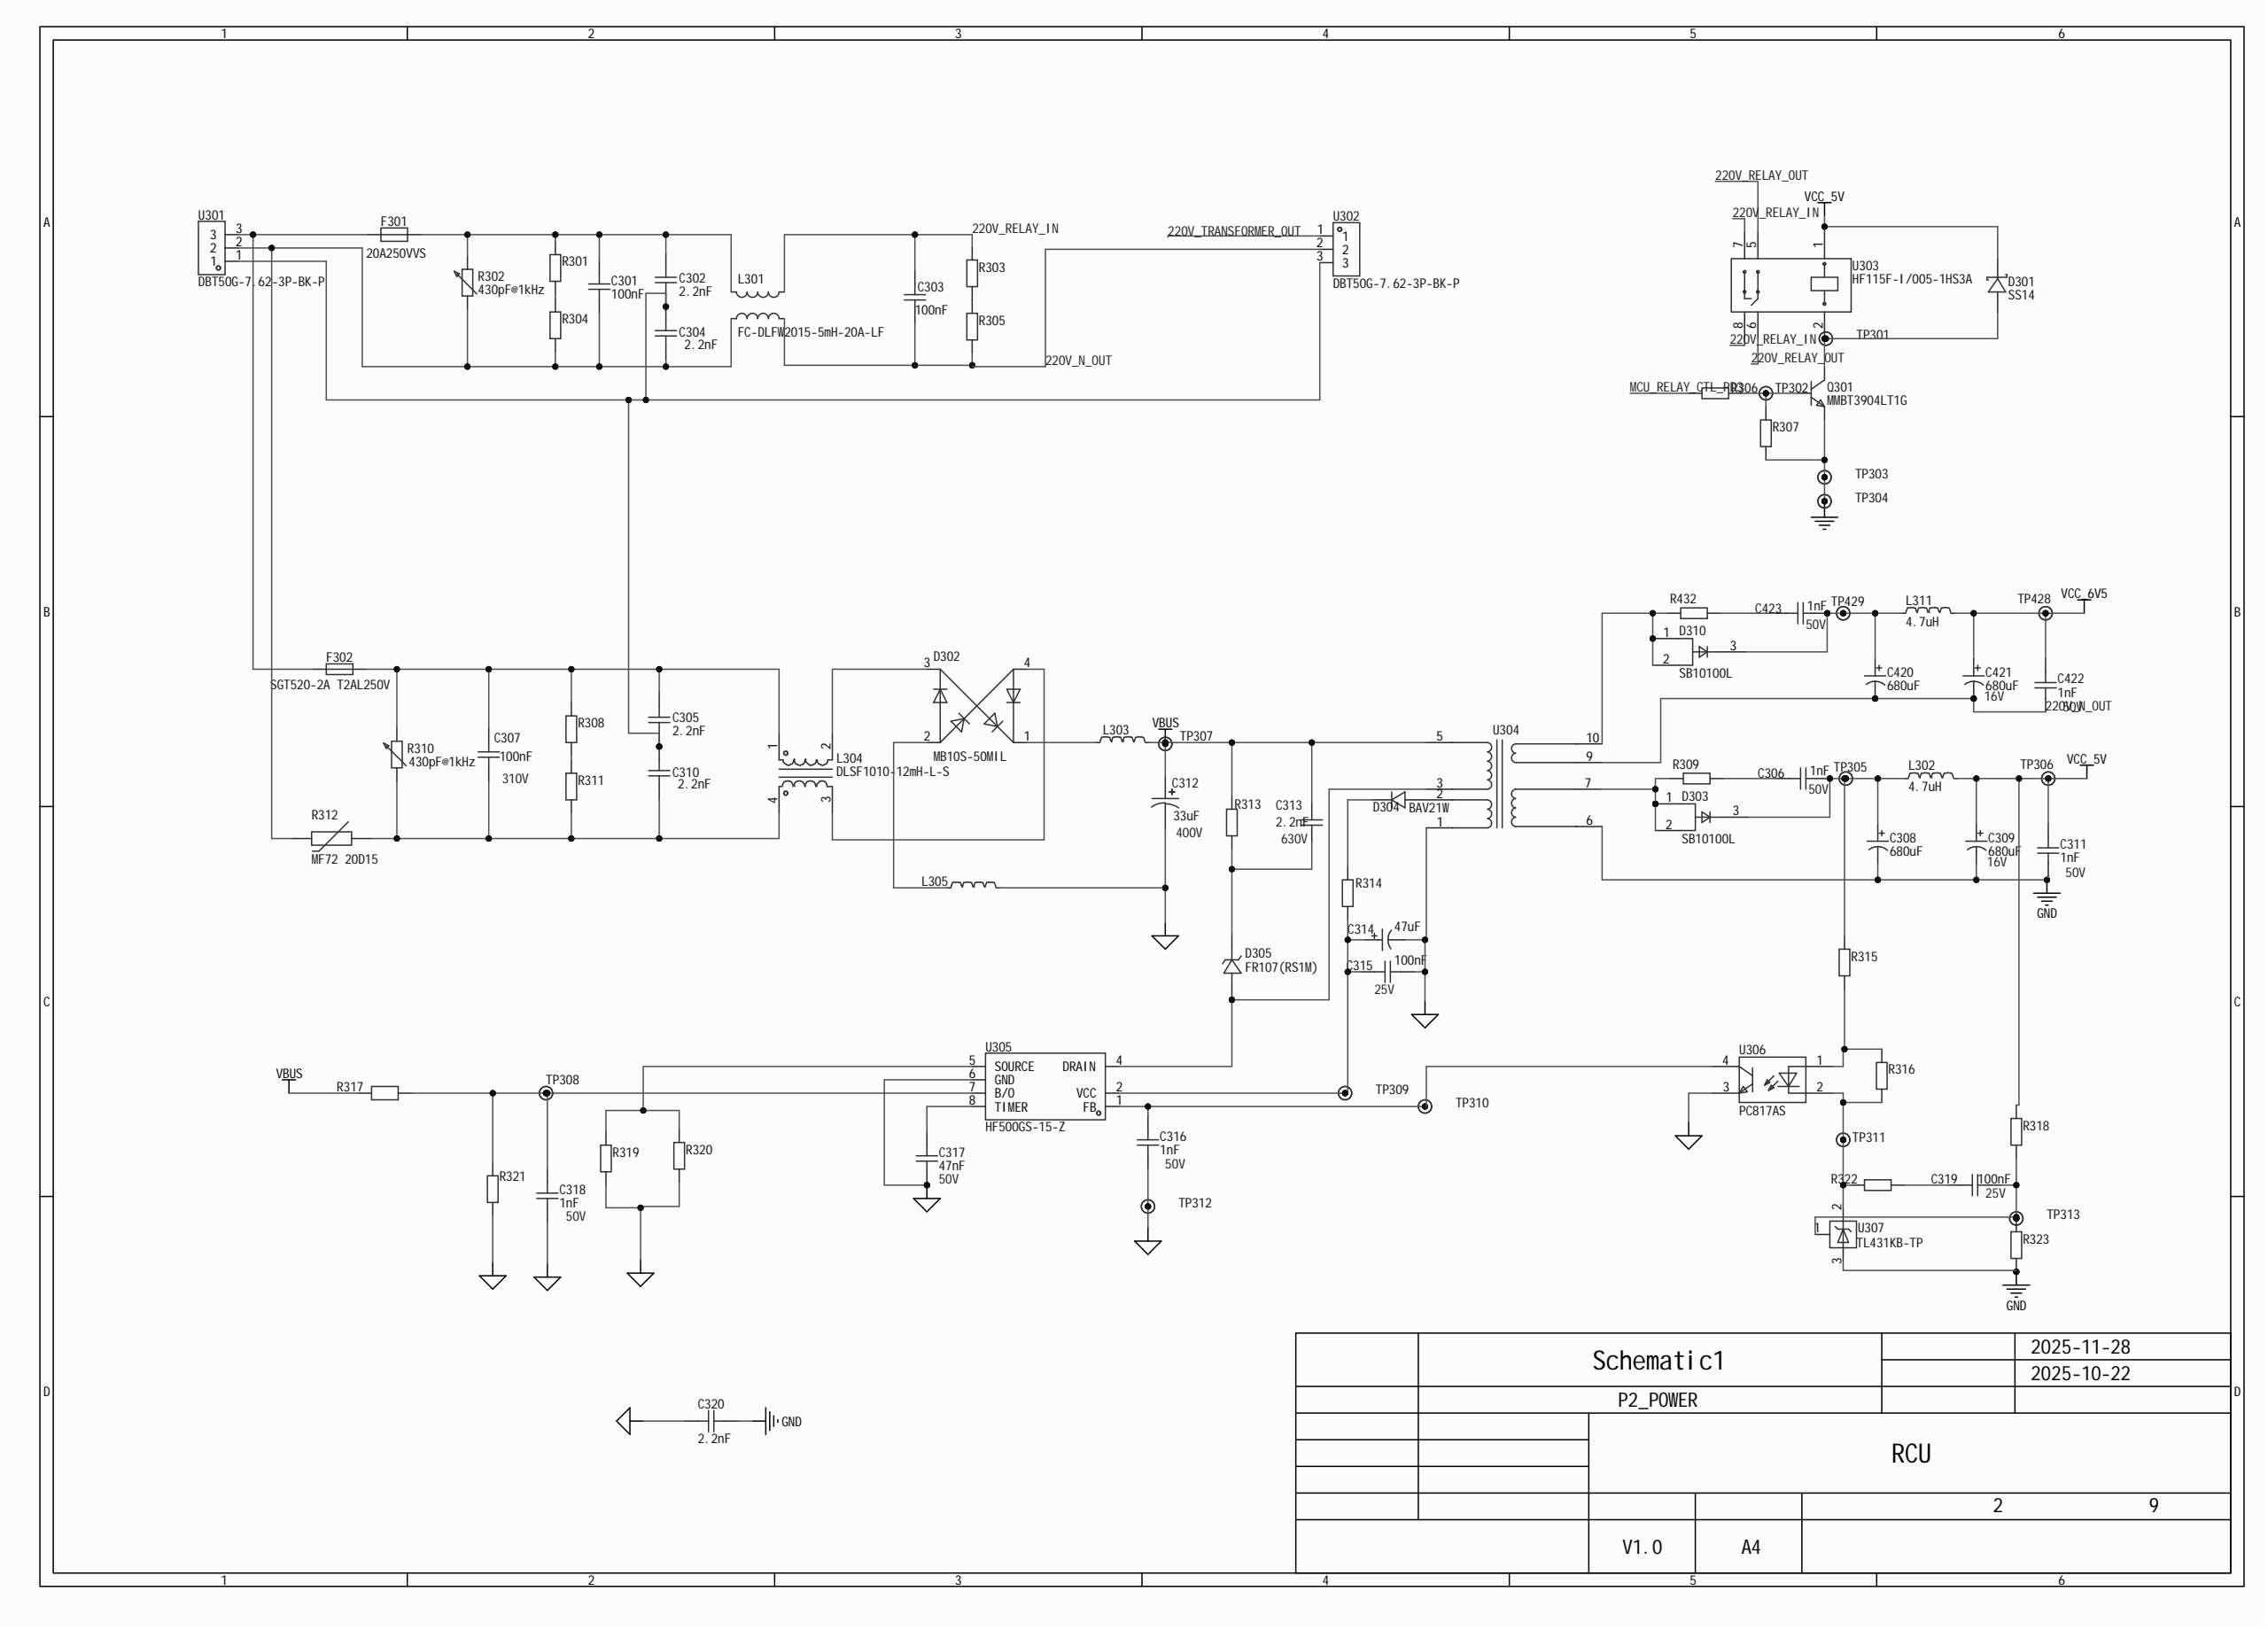Circuit board | Altium Designer | 424 parts | 202 nets | one sheet of the schematic
Parts on this sheet (reference | value | footprint):
C301 | 100nF | CAP-TH_L13.0-W6.0-P10.00-D0.6
C302 | 2.2nF | CAP-TH_L8.0-W4.0-P7.50-D1.2
C303 | 100nF | CAP-TH_L13.0-W6.0-P10.00-D0.6
C304 | 2.2nF | CAP-TH_L8.0-W4.0-P7.50-D1.2
C305 | 2.2nF | CAP-TH_L8.0-W4.0-P7.50-D1.2
C306 | 1nF | C0603
C307 | 100nF | CAP-TH_L13.0-W6.0-P10.00-D0.6
C308 | 680uF | CAP-TH_BD8.0-P3.50-D0.6-FD
C309 | 680uF | CAP-TH_BD8.0-P3.50-D0.6-FD
C310 | 2.2nF | CAP-TH_L8.0-W4.0-P7.50-D1.2
C311 | 1nF | C0603
C312 | 33uF | CAP-TH_BD10.0-P5.00-D1.0-FD
C313 | 2.2nF | C1206
C314 | 47uF | CAP-TH_BD5.0-P2.00-D0.8-FD
C315 | 100nF | C0603
C316 | 1nF | C0603
C317 | 47nF | C0603
C318 | 1nF | C0603
C319 | 100nF | C0603
C320 | 2.2nF | CAP-TH_L10.0-W4.5-P10.00-D0.6-S4.0
C420 | 680uF | CAP-TH_BD8.0-P3.50-D0.6-FD
C421 | 680uF | CAP-TH_BD8.0-P3.50-D0.6-FD
C422 | 1nF | C0603
C423 | 1nF | C0603
D301 | SS14 | SMA_L4.3-W2.6-LS5.2-RD
D302 | MB10S-50MIL | MBS_L4.7-W3.8-P2.40-LS7.0-TL
D303 | SB10100L | TO-277A_L4.7-W6.1-LS6.6-TR
D304 | BAV21W | SOD-123_L2.8-W1.8-LS3.7-RD
D305 | FR107(RS1M) | SMA_L4.3-W2.6-LS5.2-RD
D310 | SB10100L | TO-277A_L4.7-W6.1-LS6.6-TR
F301 | 20A250VVS | FUSE-TH_L8.4-W4.0-P5.08-D0.6
F302 | SGT520-2A T2AL250V | FUSE-SMD_L20.0-W5.0
L301 | FC-DLFW2015-5mH-20A-LF | FILTER-TH_FC-DLFW2015-5MH-20A-LF
L302 | 4.7uH | IND-SMD_L5.4-W5.2_FXL0530
L303 | L1206
L304 | DLSF1010-12mH-L-S | IND-TH_4P-L14.0-W12.0_DLSF1010-12MH-L-S
L305 | L1206
L311 | 4.7uH | IND-SMD_L5.4-W5.2_FXL0530
Q301 | MMBT3904LT1G | SOT-23-3_L2.9-W1.6-P1.90-LS2.8-BR
R301 | R1206
R302 | 430pF@1kHz | RES-TH_L16.5-W5.6-P7.50-D1.2-S3.00
R303 | R1206
R304 | R1206
R305 | R1206
R306 | R0603
R307 | R0603
R308 | R1206
R309 | R1206
R310 | 430pF@1kHz | RES-TH_L16.5-W5.6-P7.50-D1.2-S3.00
R311 | R1206
R312 | MF72 20D15 | RES-TH_L17.5-W6.0-P7.50-D0.8-S7.50
R313 | R1206
R314 | R1206
R315 | R0603
R316 | R0603
R317 | R1206
R318 | R0603
R319 | R1206
R320 | R1206
R321 | R0603
R322 | R0603
R323 | R0603
R432 | R1206
TP301 | Test-Point-0.5mm
TP302 | Test-Point-0.5mm
TP303 | Test-Point-0.5mm
TP304 | Test-Point-0.5mm
TP305 | Test-Point-0.5mm
TP306 | Test-Point-0.5mm
TP307 | Test-Point-0.5mm
TP308 | Test-Point-0.5mm
TP309 | Test-Point-0.5mm
TP310 | Test-Point-0.5mm
TP311 | Test-Point-0.5mm
TP312 | Test-Point-0.5mm
TP313 | Test-Point-0.5mm
TP428 | Test-Point-0.5mm
TP429 | Test-Point-0.5mm
U301 | DBT50G-7.62-3P-BK-P | CONN-TH_3P-P7.62_L15.2-W24.4-EX4.2
U302 | DBT50G-7.62-3P-BK-P | CONN-TH_3P-P7.62_L15.2-W24.4-EX4.2
U303 | HF115F-I/005-1HS3A | RELAY-TH_HF115F-XXX-1HS3
U304 | 111
U305 | HF500GS-15-Z | SOIC-8_7P-L4.9-W3.9-P1.27-LS6.0-BL-PE3
U306 | PC817AS | SOP-4_L6.5-W4.6-P2.54-LS10.2-TL
U307 | TL431KB-TP | SOT-23-3_L2.9-W1.4-P1.91-LS2.6-BR
Nets of these parts (net: part-pin ...):
VCC_6V5: C421-1 C422-2 L311-2 TP428-1
VCC_5V: C309-1 C311-2 D301-1 L302-2 R318-2 TP306-1 U303-1
VBUS: C312-1 C313-2 L303-2 R313-2 R317-1 TP307-1 U304-5
NetR319_2: R319-2 R320-2 U305-5
NetR316_1: R316-1 R322-1 TP311-1 U306-2 U307-2
NetR315_1: R315-1 R316-2 U306-1
NetR308_1: R308-1 R311-2
NetR303_1: R303-1 R305-2
NetR301_1: R301-1 R304-2
NetQ301_1: Q301-1 R306-2 R307-1 TP302-1
NetF301_1: F301-1 F302-1 U301-3
NetD310_1: D310-1 D310-2 R432-1 U304-10
NetD305_2: D305-2 U304-3 U305-4
NetD304_2: D304-2 U304-2
NetD304_1: D304-1 R314-2
NetD303_1: D303-1 D303-2 R309-1 U304-7
NetD302_4: D302-4 L304-3
NetD302_3: D302-3 L304-2
NetD302_2: D302-2 L305-1
NetD302_1: D302-1 L303-1
NetD301_2: D301-2 Q301-3 TP301-1 U303-2
NetC423_2: C423-2 R432-2
NetC420_1: C420-1 C423-1 D310-3 L311-1 TP429-1
NetC319_2: C319-2 R318-1 R323-2 TP313-1 U307-1
NetC319_1: C319-1 R322-2
NetC318_2: C318-2 R317-2 R321-2 TP308-1 U305-7
NetC317_2: C317-2 U305-8
NetC316_2: C316-2 TP310-1 U305-1 U306-4
NetC314_1: C314-1 C315-1 R314-1 TP309-1 U305-2
NetC313_1: C313-1 D305-1 R313-1
NetC307_1: C307-1 C310-1 L304-4 R310-1 R311-1 R312-2
NetC306_2: C306-2 R309-2
NetC306_1: C306-1 C308-1 D303-3 L302-1 R315-2 TP305-1
NetC305_2: C305-2 C307-2 F302-2 L304-1 R308-2 R310-2
NetC302_1: C302-1 C304-2 C305-1 C310-2 U301-1 U302-3
NetC301_2: C301-2 C302-2 F301-2 L301-2 R301-2 R302-2
NetC301_1: C301-1 C304-1 L301-1 R302-1 R304-1 R312-1 U301-2
MCU_RELAY_CTL_PD3: R306-1
GND: C308-2 C309-2 C311-1 C320-2 Q301-2 R307-2 R323-1 TP303-1 TP304-1 U304-6 U307-3
AGND: C312-2 C314-2 C315-2 C316-1 C317-1 C318-1 C320-1 L305-2 R319-1 R320-1 R321-1 TP312-1 U304-1 U305-6 U306-3
220V_TRANSFORMER_OUT: U302-1
220V_RELAY_OUT: U303-5 U303-6
220V_RELAY_IN: C303-2 L301-3 R303-2 U303-7 U303-8
220V_N_OUT: C303-1 C420-2 C421-2 C422-1 L301-4 R305-1 U302-2 U304-9